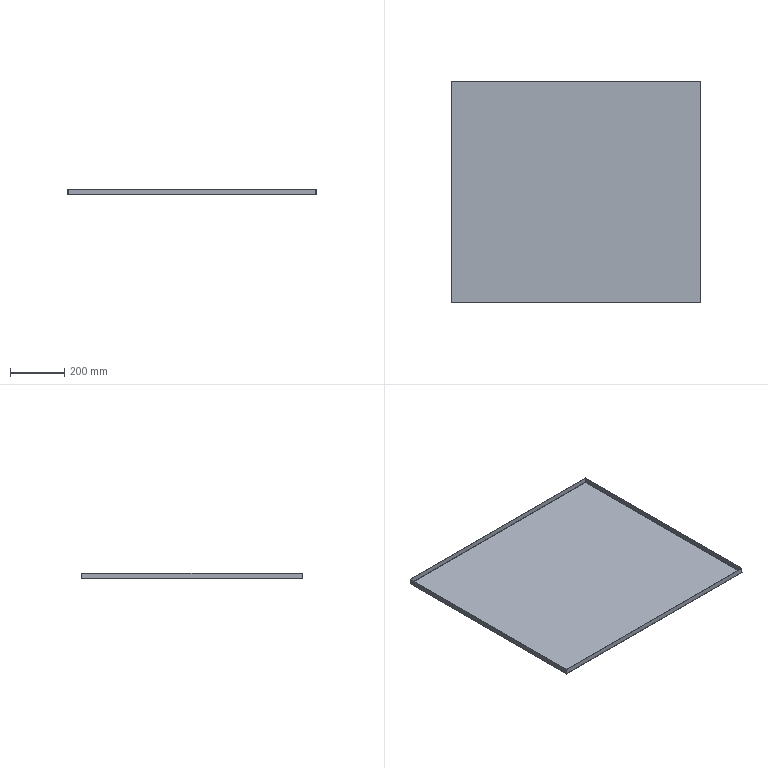Part | STEP file | Cover plate | 1 solid | 38 faces | box 918 x 818 x 20 mm | volume 977655 mm3 | plane 22 | spline 8 | cylinder 8 | commonest cylinder face diameters 0.4 x4 2.8 x4
STEP:
#1=CARTESIAN_POINT('',(457.6,-407.6,-1.2));
#2=VERTEX_POINT('',#1);
#3=CARTESIAN_POINT('',(-457.6,-407.6,-1.2));
#4=VERTEX_POINT('',#3);
#5=CARTESIAN_POINT('',(457.6,-407.6,-1.2));
#6=DIRECTION('',(-1.,0.,0.));
#7=VECTOR('',#6,1000.);
#8=LINE('',#5,#7);
#9=EDGE_CURVE('',#2,#4,#8,.T.);
#10=ORIENTED_EDGE('',*,*,#9,.T.);
#11=CARTESIAN_POINT('',(-457.6,407.6,-1.2));
#12=VERTEX_POINT('',#11);
#13=CARTESIAN_POINT('',(-457.6,-407.6,-1.2));
#14=DIRECTION('',(0.,1.,0.));
#15=VECTOR('',#14,1000.);
#16=LINE('',#13,#15);
#17=EDGE_CURVE('',#4,#12,#16,.T.);
#18=ORIENTED_EDGE('',*,*,#17,.T.);
#19=CARTESIAN_POINT('',(457.6,407.6,-1.2));
#20=VERTEX_POINT('',#19);
#21=CARTESIAN_POINT('',(-457.6,407.6,-1.2));
#22=DIRECTION('',(1.,0.,0.));
#23=VECTOR('',#22,1000.);
#24=LINE('',#21,#23);
#25=EDGE_CURVE('',#12,#20,#24,.T.);
#26=ORIENTED_EDGE('',*,*,#25,.T.);
#27=CARTESIAN_POINT('',(457.6,407.6,-1.2));
#28=DIRECTION('',(0.,-1.,0.));
#29=VECTOR('',#28,1000.);
#30=LINE('',#27,#29);
#31=EDGE_CURVE('',#20,#2,#30,.T.);
#32=ORIENTED_EDGE('',*,*,#31,.T.);
#33=EDGE_LOOP('',(#10,#18,#26,#32));
#34=FACE_OUTER_BOUND('',#33,.T.);
#35=CARTESIAN_POINT('',(0.,0.,-1.2));
#36=DIRECTION('',(0.,0.,-1.));
#37=DIRECTION('',(-1.,0.,0.));
#38=AXIS2_PLACEMENT_3D('',#35,#36,#37);
#39=PLANE('',#38);
#40=ADVANCED_FACE('',(#34),#39,.T.);
#41=CARTESIAN_POINT('',(-457.6,-407.6,0.));
#42=VERTEX_POINT('',#41);
#43=CARTESIAN_POINT('',(-457.6,407.6,0.));
#44=VERTEX_POINT('',#43);
#45=CARTESIAN_POINT('',(-457.6,-407.6,0.));
#46=DIRECTION('',(0.,1.,0.));
#47=VECTOR('',#46,1000.);
#48=LINE('',#45,#47);
#49=EDGE_CURVE('',#42,#44,#48,.T.);
#50=ORIENTED_EDGE('',*,*,#49,.F.);
#51=CARTESIAN_POINT('',(457.6,-407.6,0.));
#52=VERTEX_POINT('',#51);
#53=CARTESIAN_POINT('',(457.6,-407.6,0.));
#54=DIRECTION('',(-1.,0.,0.));
#55=VECTOR('',#54,1000.);
#56=LINE('',#53,#55);
#57=EDGE_CURVE('',#52,#42,#56,.T.);
#58=ORIENTED_EDGE('',*,*,#57,.F.);
#59=CARTESIAN_POINT('',(457.6,407.6,0.));
#60=VERTEX_POINT('',#59);
#61=CARTESIAN_POINT('',(457.6,407.6,0.));
#62=DIRECTION('',(0.,-1.,0.));
#63=VECTOR('',#62,1000.);
#64=LINE('',#61,#63);
#65=EDGE_CURVE('',#60,#52,#64,.T.);
#66=ORIENTED_EDGE('',*,*,#65,.F.);
#67=CARTESIAN_POINT('',(-457.6,407.6,0.));
#68=DIRECTION('',(1.,0.,0.));
#69=VECTOR('',#68,1000.);
#70=LINE('',#67,#69);
#71=EDGE_CURVE('',#44,#60,#70,.T.);
#72=ORIENTED_EDGE('',*,*,#71,.F.);
#73=EDGE_LOOP('',(#50,#58,#66,#72));
#74=FACE_OUTER_BOUND('',#73,.T.);
#75=CARTESIAN_POINT('',(0.,0.,0.));
#76=DIRECTION('',(0.,0.,-1.));
#77=DIRECTION('',(-1.,0.,0.));
#78=AXIS2_PLACEMENT_3D('',#75,#76,#77);
#79=PLANE('',#78);
#80=ADVANCED_FACE('',(#74),#79,.F.);
#81=CARTESIAN_POINT('',(457.093,409.,0.2));
#82=VERTEX_POINT('',#81);
#83=CARTESIAN_POINT('',(457.093,407.8,0.2));
#84=VERTEX_POINT('',#83);
#85=CARTESIAN_POINT('',(457.093,407.8,0.2));
#86=DIRECTION('',(0.,-1.,0.));
#87=VECTOR('',#86,1000.);
#88=LINE('',#85,#87);
#89=EDGE_CURVE('',#82,#84,#88,.T.);
#90=ORIENTED_EDGE('',*,*,#89,.T.);
#91=CARTESIAN_POINT('',(457.6,407.6,0.));
#92=CARTESIAN_POINT('',(457.515,407.652,0.));
#93=CARTESIAN_POINT('',(457.431,407.704,0.02155));
#94=CARTESIAN_POINT('',(457.262,407.778,0.0956));
#95=CARTESIAN_POINT('',(457.177,407.8,0.1476));
#96=CARTESIAN_POINT('',(457.093,407.8,0.2));
#97=B_SPLINE_CURVE_WITH_KNOTS('',3,(#91,#92,#93,#94,#95,#96),.UNSPECIFIED.,.F.,.F.,(4,2,4),(0.,0.5,1.),.UNSPECIFIED.);
#98=EDGE_CURVE('',#60,#84,#97,.T.);
#99=ORIENTED_EDGE('',*,*,#98,.F.);
#100=CARTESIAN_POINT('',(457.6,407.6,0.));
#101=DIRECTION('',(0.,0.,-1.));
#102=VECTOR('',#101,1000.);
#103=LINE('',#100,#102);
#104=EDGE_CURVE('',#60,#20,#103,.T.);
#105=ORIENTED_EDGE('',*,*,#104,.T.);
#106=CARTESIAN_POINT('',(457.6,407.6,-1.2));
#107=CARTESIAN_POINT('',(457.558,407.783,-1.2));
#108=CARTESIAN_POINT('',(457.515,407.966,-1.164));
#109=CARTESIAN_POINT('',(457.431,408.305,-1.023));
#110=CARTESIAN_POINT('',(457.389,408.46,-0.9195));
#111=CARTESIAN_POINT('',(457.304,408.72,-0.6604));
#112=CARTESIAN_POINT('',(457.262,408.823,-0.5051));
#113=CARTESIAN_POINT('',(457.177,408.964,-0.1664));
#114=CARTESIAN_POINT('',(457.135,409.,0.01674));
#115=CARTESIAN_POINT('',(457.093,409.,0.2));
#116=B_SPLINE_CURVE_WITH_KNOTS('',3,(#106,#107,#108,#109,#110,#111,#112,#113,#114,#115),.UNSPECIFIED.,.F.,.F.,(4,2,2,2,4),(0.,0.25,0.5,0.75,1.),.UNSPECIFIED.);
#117=EDGE_CURVE('',#20,#82,#116,.T.);
#118=ORIENTED_EDGE('',*,*,#117,.T.);
#119=EDGE_LOOP('',(#90,#99,#105,#118));
#120=FACE_OUTER_BOUND('',#119,.T.);
#121=CARTESIAN_POINT('',(457.6,407.6,-1.212));
#122=CARTESIAN_POINT('',(457.558,407.785,-1.212));
#123=CARTESIAN_POINT('',(457.515,407.97,-1.175));
#124=CARTESIAN_POINT('',(457.431,408.311,-1.034));
#125=CARTESIAN_POINT('',(457.389,408.468,-0.9291));
#126=CARTESIAN_POINT('',(457.304,408.729,-0.6677));
#127=CARTESIAN_POINT('',(457.262,408.834,-0.5111));
#128=CARTESIAN_POINT('',(457.177,408.975,-0.1696));
#129=CARTESIAN_POINT('',(457.135,409.012,0.01514));
#130=CARTESIAN_POINT('',(457.093,409.012,0.2));
#131=CARTESIAN_POINT('',(457.6,407.6,-1.2));
#132=CARTESIAN_POINT('',(457.558,407.783,-1.2));
#133=CARTESIAN_POINT('',(457.515,407.966,-1.164));
#134=CARTESIAN_POINT('',(457.431,408.305,-1.023));
#135=CARTESIAN_POINT('',(457.389,408.46,-0.9195));
#136=CARTESIAN_POINT('',(457.304,408.72,-0.6604));
#137=CARTESIAN_POINT('',(457.262,408.823,-0.5051));
#138=CARTESIAN_POINT('',(457.177,408.964,-0.1664));
#139=CARTESIAN_POINT('',(457.135,409.,0.01671));
#140=CARTESIAN_POINT('',(457.093,409.,0.2));
#141=CARTESIAN_POINT('',(457.6,407.6,0.));
#142=CARTESIAN_POINT('',(457.558,407.626,0.));
#143=CARTESIAN_POINT('',(457.515,407.652,0.005205));
#144=CARTESIAN_POINT('',(457.431,407.701,0.02524));
#145=CARTESIAN_POINT('',(457.389,407.723,0.04007));
#146=CARTESIAN_POINT('',(457.304,407.76,0.07709));
#147=CARTESIAN_POINT('',(457.262,407.775,0.09928));
#148=CARTESIAN_POINT('',(457.177,407.795,0.1477));
#149=CARTESIAN_POINT('',(457.135,407.8,0.1738));
#150=CARTESIAN_POINT('',(457.093,407.8,0.2));
#151=CARTESIAN_POINT('',(457.6,407.6,0.01212));
#152=CARTESIAN_POINT('',(457.558,407.625,0.01212));
#153=CARTESIAN_POINT('',(457.515,407.649,0.01701));
#154=CARTESIAN_POINT('',(457.431,407.695,0.03583));
#155=CARTESIAN_POINT('',(457.389,407.715,0.04976));
#156=CARTESIAN_POINT('',(457.304,407.75,0.08454));
#157=CARTESIAN_POINT('',(457.262,407.764,0.1054));
#158=CARTESIAN_POINT('',(457.177,407.783,0.1508));
#159=CARTESIAN_POINT('',(457.135,407.788,0.1754));
#160=CARTESIAN_POINT('',(457.093,407.788,0.2));
#161=B_SPLINE_SURFACE_WITH_KNOTS('',1,3,((#121,#122,#123,#124,#125,#126,#127,#128,#129,#130),(#131,#132,#133,#134,#135,#136,#137,#138,#139,#140),(#141,#142,#143,#144,#145,#146,#147,#148,#149,#150),(#151,#152,#153,#154,#155,#156,#157,#158,#159,#160)),.UNSPECIFIED.,.F.,.F.,.F.,(2,1,1,2),(4,2,2,2,4),(-0.01,0.,1.,1.01),(0.,0.25,0.5,0.75,1.),.UNSPECIFIED.);
#162=ADVANCED_FACE('',(#120),#161,.F.);
#163=CARTESIAN_POINT('',(-457.093,407.8,0.2));
#164=VERTEX_POINT('',#163);
#165=CARTESIAN_POINT('',(-457.093,407.8,0.2));
#166=CARTESIAN_POINT('',(-457.177,407.8,0.1476));
#167=CARTESIAN_POINT('',(-457.262,407.778,0.0956));
#168=CARTESIAN_POINT('',(-457.431,407.704,0.02155));
#169=CARTESIAN_POINT('',(-457.515,407.652,0.));
#170=CARTESIAN_POINT('',(-457.6,407.6,0.));
#171=B_SPLINE_CURVE_WITH_KNOTS('',3,(#165,#166,#167,#168,#169,#170),.UNSPECIFIED.,.F.,.F.,(4,2,4),(0.,0.5,1.),.UNSPECIFIED.);
#172=EDGE_CURVE('',#164,#44,#171,.T.);
#173=ORIENTED_EDGE('',*,*,#172,.F.);
#174=CARTESIAN_POINT('',(-457.093,409.,0.2));
#175=VERTEX_POINT('',#174);
#176=CARTESIAN_POINT('',(-457.093,407.8,0.2));
#177=DIRECTION('',(0.,-1.,0.));
#178=VECTOR('',#177,1000.);
#179=LINE('',#176,#178);
#180=EDGE_CURVE('',#175,#164,#179,.T.);
#181=ORIENTED_EDGE('',*,*,#180,.F.);
#182=CARTESIAN_POINT('',(-457.093,409.,0.2));
#183=CARTESIAN_POINT('',(-457.135,409.,0.01674));
#184=CARTESIAN_POINT('',(-457.177,408.964,-0.1664));
#185=CARTESIAN_POINT('',(-457.262,408.823,-0.5051));
#186=CARTESIAN_POINT('',(-457.304,408.72,-0.6604));
#187=CARTESIAN_POINT('',(-457.389,408.46,-0.9195));
#188=CARTESIAN_POINT('',(-457.431,408.305,-1.023));
#189=CARTESIAN_POINT('',(-457.515,407.966,-1.164));
#190=CARTESIAN_POINT('',(-457.558,407.783,-1.2));
#191=CARTESIAN_POINT('',(-457.6,407.6,-1.2));
#192=B_SPLINE_CURVE_WITH_KNOTS('',3,(#182,#183,#184,#185,#186,#187,#188,#189,#190,#191),.UNSPECIFIED.,.F.,.F.,(4,2,2,2,4),(0.,0.25,0.5,0.75,1.),.UNSPECIFIED.);
#193=EDGE_CURVE('',#175,#12,#192,.T.);
#194=ORIENTED_EDGE('',*,*,#193,.T.);
#195=CARTESIAN_POINT('',(-457.6,407.6,0.));
#196=DIRECTION('',(0.,0.,-1.));
#197=VECTOR('',#196,1000.);
#198=LINE('',#195,#197);
#199=EDGE_CURVE('',#44,#12,#198,.T.);
#200=ORIENTED_EDGE('',*,*,#199,.F.);
#201=EDGE_LOOP('',(#173,#181,#194,#200));
#202=FACE_OUTER_BOUND('',#201,.T.);
#203=CARTESIAN_POINT('',(-457.093,409.012,0.2));
#204=CARTESIAN_POINT('',(-457.135,409.012,0.01514));
#205=CARTESIAN_POINT('',(-457.177,408.975,-0.1696));
#206=CARTESIAN_POINT('',(-457.262,408.834,-0.5111));
#207=CARTESIAN_POINT('',(-457.304,408.729,-0.6677));
#208=CARTESIAN_POINT('',(-457.389,408.468,-0.9291));
#209=CARTESIAN_POINT('',(-457.431,408.311,-1.034));
#210=CARTESIAN_POINT('',(-457.515,407.97,-1.175));
#211=CARTESIAN_POINT('',(-457.558,407.785,-1.212));
#212=CARTESIAN_POINT('',(-457.6,407.6,-1.212));
#213=CARTESIAN_POINT('',(-457.093,409.,0.2));
#214=CARTESIAN_POINT('',(-457.135,409.,0.01671));
#215=CARTESIAN_POINT('',(-457.177,408.964,-0.1664));
#216=CARTESIAN_POINT('',(-457.262,408.823,-0.5051));
#217=CARTESIAN_POINT('',(-457.304,408.72,-0.6604));
#218=CARTESIAN_POINT('',(-457.389,408.46,-0.9195));
#219=CARTESIAN_POINT('',(-457.431,408.305,-1.023));
#220=CARTESIAN_POINT('',(-457.515,407.966,-1.164));
#221=CARTESIAN_POINT('',(-457.558,407.783,-1.2));
#222=CARTESIAN_POINT('',(-457.6,407.6,-1.2));
#223=CARTESIAN_POINT('',(-457.093,407.8,0.2));
#224=CARTESIAN_POINT('',(-457.135,407.8,0.1738));
#225=CARTESIAN_POINT('',(-457.177,407.795,0.1477));
#226=CARTESIAN_POINT('',(-457.262,407.775,0.09928));
#227=CARTESIAN_POINT('',(-457.304,407.76,0.07709));
#228=CARTESIAN_POINT('',(-457.389,407.723,0.04007));
#229=CARTESIAN_POINT('',(-457.431,407.701,0.02524));
#230=CARTESIAN_POINT('',(-457.515,407.652,0.005205));
#231=CARTESIAN_POINT('',(-457.558,407.626,0.));
#232=CARTESIAN_POINT('',(-457.6,407.6,0.));
#233=CARTESIAN_POINT('',(-457.093,407.788,0.2));
#234=CARTESIAN_POINT('',(-457.135,407.788,0.1754));
#235=CARTESIAN_POINT('',(-457.177,407.783,0.1508));
#236=CARTESIAN_POINT('',(-457.262,407.764,0.1054));
#237=CARTESIAN_POINT('',(-457.304,407.75,0.08454));
#238=CARTESIAN_POINT('',(-457.389,407.715,0.04976));
#239=CARTESIAN_POINT('',(-457.431,407.695,0.03583));
#240=CARTESIAN_POINT('',(-457.515,407.649,0.01701));
#241=CARTESIAN_POINT('',(-457.558,407.625,0.01212));
#242=CARTESIAN_POINT('',(-457.6,407.6,0.01212));
#243=B_SPLINE_SURFACE_WITH_KNOTS('',1,3,((#203,#204,#205,#206,#207,#208,#209,#210,#211,#212),(#213,#214,#215,#216,#217,#218,#219,#220,#221,#222),(#223,#224,#225,#226,#227,#228,#229,#230,#231,#232),(#233,#234,#235,#236,#237,#238,#239,#240,#241,#242)),.UNSPECIFIED.,.F.,.F.,.F.,(2,1,1,2),(4,2,2,2,4),(-0.01,0.,1.,1.01),(0.,0.25,0.5,0.75,1.),.UNSPECIFIED.);
#244=ADVANCED_FACE('',(#202),#243,.F.);
#245=ORIENTED_EDGE('',*,*,#25,.F.);
#246=ORIENTED_EDGE('',*,*,#193,.F.);
#247=CARTESIAN_POINT('',(459.,409.,0.2));
#248=DIRECTION('',(1.,0.,0.));
#249=VECTOR('',#248,1000.);
#250=LINE('',#247,#249);
#251=EDGE_CURVE('',#175,#82,#250,.T.);
#252=ORIENTED_EDGE('',*,*,#251,.T.);
#253=ORIENTED_EDGE('',*,*,#117,.F.);
#254=EDGE_LOOP('',(#245,#246,#252,#253));
#255=FACE_OUTER_BOUND('',#254,.T.);
#256=CARTESIAN_POINT('',(-457.6,407.6,0.2));
#257=DIRECTION('',(-1.,0.,0.));
#258=DIRECTION('',(0.,1.,0.));
#259=AXIS2_PLACEMENT_3D('',#256,#257,#258);
#260=CYLINDRICAL_SURFACE('',#259,1.4);
#261=ADVANCED_FACE('',(#255),#260,.T.);
#262=ORIENTED_EDGE('',*,*,#71,.T.);
#263=ORIENTED_EDGE('',*,*,#98,.T.);
#264=CARTESIAN_POINT('',(459.,407.8,0.2));
#265=DIRECTION('',(-1.,0.,0.));
#266=VECTOR('',#265,1000.);
#267=LINE('',#264,#266);
#268=EDGE_CURVE('',#84,#164,#267,.T.);
#269=ORIENTED_EDGE('',*,*,#268,.T.);
#270=ORIENTED_EDGE('',*,*,#172,.T.);
#271=EDGE_LOOP('',(#262,#263,#269,#270));
#272=FACE_OUTER_BOUND('',#271,.T.);
#273=CARTESIAN_POINT('',(-457.6,407.6,0.2));
#274=DIRECTION('',(-1.,0.,0.));
#275=DIRECTION('',(0.,1.,0.));
#276=AXIS2_PLACEMENT_3D('',#273,#274,#275);
#277=CYLINDRICAL_SURFACE('',#276,0.2);
#278=ADVANCED_FACE('',(#272),#277,.F.);
#279=CARTESIAN_POINT('',(457.093,409.,18.8));
#280=VERTEX_POINT('',#279);
#281=CARTESIAN_POINT('',(457.093,409.,0.));
#282=DIRECTION('',(0.,0.,1.));
#283=VECTOR('',#282,1000.);
#284=LINE('',#281,#283);
#285=EDGE_CURVE('',#82,#280,#284,.T.);
#286=ORIENTED_EDGE('',*,*,#285,.T.);
#287=CARTESIAN_POINT('',(457.093,407.8,18.8));
#288=VERTEX_POINT('',#287);
#289=CARTESIAN_POINT('',(457.093,407.8,18.8));
#290=DIRECTION('',(0.,-1.,0.));
#291=VECTOR('',#290,1000.);
#292=LINE('',#289,#291);
#293=EDGE_CURVE('',#280,#288,#292,.T.);
#294=ORIENTED_EDGE('',*,*,#293,.T.);
#295=CARTESIAN_POINT('',(457.093,407.8,0.));
#296=DIRECTION('',(0.,0.,1.));
#297=VECTOR('',#296,1000.);
#298=LINE('',#295,#297);
#299=EDGE_CURVE('',#84,#288,#298,.T.);
#300=ORIENTED_EDGE('',*,*,#299,.F.);
#301=ORIENTED_EDGE('',*,*,#89,.F.);
#302=EDGE_LOOP('',(#286,#294,#300,#301));
#303=FACE_OUTER_BOUND('',#302,.T.);
#304=CARTESIAN_POINT('',(457.093,407.8,0.));
#305=DIRECTION('',(1.,0.,0.));
#306=DIRECTION('',(0.,0.,-1.));
#307=AXIS2_PLACEMENT_3D('',#304,#305,#306);
#308=PLANE('',#307);
#309=ADVANCED_FACE('',(#303),#308,.T.);
#310=ORIENTED_EDGE('',*,*,#251,.F.);
#311=CARTESIAN_POINT('',(-457.093,409.,18.8));
#312=VERTEX_POINT('',#311);
#313=CARTESIAN_POINT('',(-457.093,409.,0.));
#314=DIRECTION('',(0.,0.,1.));
#315=VECTOR('',#314,1000.);
#316=LINE('',#313,#315);
#317=EDGE_CURVE('',#175,#312,#316,.T.);
#318=ORIENTED_EDGE('',*,*,#317,.T.);
#319=CARTESIAN_POINT('',(0.,409.,18.8));
#320=DIRECTION('',(1.,0.,0.));
#321=VECTOR('',#320,1000.);
#322=LINE('',#319,#321);
#323=EDGE_CURVE('',#312,#280,#322,.T.);
#324=ORIENTED_EDGE('',*,*,#323,.T.);
#325=ORIENTED_EDGE('',*,*,#285,.F.);
#326=EDGE_LOOP('',(#310,#318,#324,#325));
#327=FACE_OUTER_BOUND('',#326,.T.);
#328=CARTESIAN_POINT('',(0.,409.,0.));
#329=DIRECTION('',(0.,-1.,0.));
#330=DIRECTION('',(0.,0.,-1.));
#331=AXIS2_PLACEMENT_3D('',#328,#329,#330);
#332=PLANE('',#331);
#333=ADVANCED_FACE('',(#327),#332,.F.);
#334=CARTESIAN_POINT('',(-457.093,407.8,18.8));
#335=VERTEX_POINT('',#334);
#336=CARTESIAN_POINT('',(-457.093,407.8,0.));
#337=DIRECTION('',(0.,0.,1.));
#338=VECTOR('',#337,1000.);
#339=LINE('',#336,#338);
#340=EDGE_CURVE('',#164,#335,#339,.T.);
#341=ORIENTED_EDGE('',*,*,#340,.F.);
#342=ORIENTED_EDGE('',*,*,#268,.F.);
#343=ORIENTED_EDGE('',*,*,#299,.T.);
#344=CARTESIAN_POINT('',(459.,407.8,18.8));
#345=DIRECTION('',(1.,0.,0.));
#346=VECTOR('',#345,1000.);
#347=LINE('',#344,#346);
#348=EDGE_CURVE('',#335,#288,#347,.T.);
#349=ORIENTED_EDGE('',*,*,#348,.F.);
#350=EDGE_LOOP('',(#341,#342,#343,#349));
#351=FACE_OUTER_BOUND('',#350,.T.);
#352=CARTESIAN_POINT('',(0.,407.8,0.));
#353=DIRECTION('',(0.,-1.,0.));
#354=DIRECTION('',(0.,0.,-1.));
#355=AXIS2_PLACEMENT_3D('',#352,#353,#354);
#356=PLANE('',#355);
#357=ADVANCED_FACE('',(#351),#356,.T.);
#358=ORIENTED_EDGE('',*,*,#323,.F.);
#359=CARTESIAN_POINT('',(-457.093,409.,18.8));
#360=DIRECTION('',(0.,-1.,0.));
#361=VECTOR('',#360,1000.);
#362=LINE('',#359,#361);
#363=EDGE_CURVE('',#312,#335,#362,.T.);
#364=ORIENTED_EDGE('',*,*,#363,.T.);
#365=ORIENTED_EDGE('',*,*,#348,.T.);
#366=ORIENTED_EDGE('',*,*,#293,.F.);
#367=EDGE_LOOP('',(#358,#364,#365,#366));
#368=FACE_OUTER_BOUND('',#367,.T.);
#369=CARTESIAN_POINT('',(459.,409.,18.8));
#370=DIRECTION('',(0.,0.,-1.));
#371=DIRECTION('',(0.,1.,0.));
#372=AXIS2_PLACEMENT_3D('',#369,#370,#371);
#373=PLANE('',#372);
#374=ADVANCED_FACE('',(#368),#373,.F.);
#375=ORIENTED_EDGE('',*,*,#363,.F.);
#376=ORIENTED_EDGE('',*,*,#317,.F.);
#377=ORIENTED_EDGE('',*,*,#180,.T.);
#378=ORIENTED_EDGE('',*,*,#340,.T.);
#379=EDGE_LOOP('',(#375,#376,#377,#378));
#380=FACE_OUTER_BOUND('',#379,.T.);
#381=CARTESIAN_POINT('',(-457.093,407.8,0.));
#382=DIRECTION('',(1.,0.,0.));
#383=DIRECTION('',(0.,0.,-1.));
#384=AXIS2_PLACEMENT_3D('',#381,#382,#383);
#385=PLANE('',#384);
#386=ADVANCED_FACE('',(#380),#385,.F.);
#387=CARTESIAN_POINT('',(459.,-407.093,0.2));
#388=VERTEX_POINT('',#387);
#389=CARTESIAN_POINT('',(457.8,-407.093,0.2));
#390=VERTEX_POINT('',#389);
#391=CARTESIAN_POINT('',(457.8,-407.093,0.2));
#392=DIRECTION('',(-1.,0.,0.));
#393=VECTOR('',#392,1000.);
#394=LINE('',#391,#393);
#395=EDGE_CURVE('',#388,#390,#394,.T.);
#396=ORIENTED_EDGE('',*,*,#395,.T.);
#397=CARTESIAN_POINT('',(457.6,-407.6,0.));
#398=CARTESIAN_POINT('',(457.652,-407.515,0.));
#399=CARTESIAN_POINT('',(457.704,-407.431,0.02155));
#400=CARTESIAN_POINT('',(457.778,-407.262,0.0956));
#401=CARTESIAN_POINT('',(457.8,-407.177,0.1476));
#402=CARTESIAN_POINT('',(457.8,-407.093,0.2));
#403=B_SPLINE_CURVE_WITH_KNOTS('',3,(#397,#398,#399,#400,#401,#402),.UNSPECIFIED.,.F.,.F.,(4,2,4),(0.,0.5,1.),.UNSPECIFIED.);
#404=EDGE_CURVE('',#52,#390,#403,.T.);
#405=ORIENTED_EDGE('',*,*,#404,.F.);
#406=CARTESIAN_POINT('',(457.6,-407.6,0.));
#407=DIRECTION('',(0.,0.,-1.));
#408=VECTOR('',#407,1000.);
#409=LINE('',#406,#408);
#410=EDGE_CURVE('',#52,#2,#409,.T.);
#411=ORIENTED_EDGE('',*,*,#410,.T.);
#412=CARTESIAN_POINT('',(457.6,-407.6,-1.2));
#413=CARTESIAN_POINT('',(457.783,-407.558,-1.2));
#414=CARTESIAN_POINT('',(457.966,-407.515,-1.164));
#415=CARTESIAN_POINT('',(458.305,-407.431,-1.023));
#416=CARTESIAN_POINT('',(458.46,-407.389,-0.9195));
#417=CARTESIAN_POINT('',(458.72,-407.304,-0.6604));
#418=CARTESIAN_POINT('',(458.823,-407.262,-0.5051));
#419=CARTESIAN_POINT('',(458.964,-407.177,-0.1664));
#420=CARTESIAN_POINT('',(459.,-407.135,0.01674));
#421=CARTESIAN_POINT('',(459.,-407.093,0.2));
#422=B_SPLINE_CURVE_WITH_KNOTS('',3,(#412,#413,#414,#415,#416,#417,#418,#419,#420,#421),.UNSPECIFIED.,.F.,.F.,(4,2,2,2,4),(0.,0.25,0.5,0.75,1.),.UNSPECIFIED.);
#423=EDGE_CURVE('',#2,#388,#422,.T.);
#424=ORIENTED_EDGE('',*,*,#423,.T.);
#425=EDGE_LOOP('',(#396,#405,#411,#424));
#426=FACE_OUTER_BOUND('',#425,.T.);
#427=CARTESIAN_POINT('',(457.6,-407.6,-1.212));
#428=CARTESIAN_POINT('',(457.785,-407.558,-1.212));
#429=CARTESIAN_POINT('',(457.97,-407.515,-1.175));
#430=CARTESIAN_POINT('',(458.311,-407.431,-1.034));
#431=CARTESIAN_POINT('',(458.468,-407.389,-0.9291));
#432=CARTESIAN_POINT('',(458.729,-407.304,-0.6677));
#433=CARTESIAN_POINT('',(458.834,-407.262,-0.5111));
#434=CARTESIAN_POINT('',(458.975,-407.177,-0.1696));
#435=CARTESIAN_POINT('',(459.012,-407.135,0.01514));
#436=CARTESIAN_POINT('',(459.012,-407.093,0.2));
#437=CARTESIAN_POINT('',(457.6,-407.6,-1.2));
#438=CARTESIAN_POINT('',(457.783,-407.558,-1.2));
#439=CARTESIAN_POINT('',(457.966,-407.515,-1.164));
#440=CARTESIAN_POINT('',(458.305,-407.431,-1.023));
#441=CARTESIAN_POINT('',(458.46,-407.389,-0.9195));
#442=CARTESIAN_POINT('',(458.72,-407.304,-0.6604));
#443=CARTESIAN_POINT('',(458.823,-407.262,-0.5051));
#444=CARTESIAN_POINT('',(458.964,-407.177,-0.1664));
#445=CARTESIAN_POINT('',(459.,-407.135,0.01671));
#446=CARTESIAN_POINT('',(459.,-407.093,0.2));
#447=CARTESIAN_POINT('',(457.6,-407.6,0.));
#448=CARTESIAN_POINT('',(457.626,-407.558,0.));
#449=CARTESIAN_POINT('',(457.652,-407.515,0.005205));
#450=CARTESIAN_POINT('',(457.701,-407.431,0.02524));
#451=CARTESIAN_POINT('',(457.723,-407.389,0.04007));
#452=CARTESIAN_POINT('',(457.76,-407.304,0.07709));
#453=CARTESIAN_POINT('',(457.775,-407.262,0.09928));
#454=CARTESIAN_POINT('',(457.795,-407.177,0.1477));
#455=CARTESIAN_POINT('',(457.8,-407.135,0.1738));
#456=CARTESIAN_POINT('',(457.8,-407.093,0.2));
#457=CARTESIAN_POINT('',(457.6,-407.6,0.01212));
#458=CARTESIAN_POINT('',(457.625,-407.558,0.01212));
#459=CARTESIAN_POINT('',(457.649,-407.515,0.01701));
#460=CARTESIAN_POINT('',(457.695,-407.431,0.03583));
#461=CARTESIAN_POINT('',(457.715,-407.389,0.04976));
#462=CARTESIAN_POINT('',(457.75,-407.304,0.08454));
#463=CARTESIAN_POINT('',(457.764,-407.262,0.1054));
#464=CARTESIAN_POINT('',(457.783,-407.177,0.1508));
#465=CARTESIAN_POINT('',(457.788,-407.135,0.1754));
#466=CARTESIAN_POINT('',(457.788,-407.093,0.2));
#467=B_SPLINE_SURFACE_WITH_KNOTS('',1,3,((#427,#428,#429,#430,#431,#432,#433,#434,#435,#436),(#437,#438,#439,#440,#441,#442,#443,#444,#445,#446),(#447,#448,#449,#450,#451,#452,#453,#454,#455,#456),(#457,#458,#459,#460,#461,#462,#463,#464,#465,#466)),.UNSPECIFIED.,.F.,.F.,.F.,(2,1,1,2),(4,2,2,2,4),(-0.01,0.,1.,1.01),(0.,0.25,0.5,0.75,1.),.UNSPECIFIED.);
#468=ADVANCED_FACE('',(#426),#467,.F.);
#469=CARTESIAN_POINT('',(457.8,407.093,0.2));
#470=VERTEX_POINT('',#469);
#471=CARTESIAN_POINT('',(457.8,407.093,0.2));
#472=CARTESIAN_POINT('',(457.8,407.177,0.1476));
#473=CARTESIAN_POINT('',(457.778,407.262,0.0956));
#474=CARTESIAN_POINT('',(457.704,407.431,0.02155));
#475=CARTESIAN_POINT('',(457.652,407.515,0.));
#476=CARTESIAN_POINT('',(457.6,407.6,0.));
#477=B_SPLINE_CURVE_WITH_KNOTS('',3,(#471,#472,#473,#474,#475,#476),.UNSPECIFIED.,.F.,.F.,(4,2,4),(0.,0.5,1.),.UNSPECIFIED.);
#478=EDGE_CURVE('',#470,#60,#477,.T.);
#479=ORIENTED_EDGE('',*,*,#478,.F.);
#480=CARTESIAN_POINT('',(459.,407.093,0.2));
#481=VERTEX_POINT('',#480);
#482=CARTESIAN_POINT('',(457.8,407.093,0.2));
#483=DIRECTION('',(-1.,0.,0.));
#484=VECTOR('',#483,1000.);
#485=LINE('',#482,#484);
#486=EDGE_CURVE('',#481,#470,#485,.T.);
#487=ORIENTED_EDGE('',*,*,#486,.F.);
#488=CARTESIAN_POINT('',(459.,407.093,0.2));
#489=CARTESIAN_POINT('',(459.,407.135,0.01674));
#490=CARTESIAN_POINT('',(458.964,407.177,-0.1664));
#491=CARTESIAN_POINT('',(458.823,407.262,-0.5051));
#492=CARTESIAN_POINT('',(458.72,407.304,-0.6604));
#493=CARTESIAN_POINT('',(458.46,407.389,-0.9195));
#494=CARTESIAN_POINT('',(458.305,407.431,-1.023));
#495=CARTESIAN_POINT('',(457.966,407.515,-1.164));
#496=CARTESIAN_POINT('',(457.783,407.558,-1.2));
#497=CARTESIAN_POINT('',(457.6,407.6,-1.2));
#498=B_SPLINE_CURVE_WITH_KNOTS('',3,(#488,#489,#490,#491,#492,#493,#494,#495,#496,#497),.UNSPECIFIED.,.F.,.F.,(4,2,2,2,4),(0.,0.25,0.5,0.75,1.),.UNSPECIFIED.);
#499=EDGE_CURVE('',#481,#20,#498,.T.);
#500=ORIENTED_EDGE('',*,*,#499,.T.);
#501=ORIENTED_EDGE('',*,*,#104,.F.);
#502=EDGE_LOOP('',(#479,#487,#500,#501));
#503=FACE_OUTER_BOUND('',#502,.T.);
#504=CARTESIAN_POINT('',(459.012,407.093,0.2));
#505=CARTESIAN_POINT('',(459.012,407.135,0.01514));
#506=CARTESIAN_POINT('',(458.975,407.177,-0.1696));
#507=CARTESIAN_POINT('',(458.834,407.262,-0.5111));
#508=CARTESIAN_POINT('',(458.729,407.304,-0.6677));
#509=CARTESIAN_POINT('',(458.468,407.389,-0.9291));
#510=CARTESIAN_POINT('',(458.311,407.431,-1.034));
#511=CARTESIAN_POINT('',(457.97,407.515,-1.175));
#512=CARTESIAN_POINT('',(457.785,407.558,-1.212));
#513=CARTESIAN_POINT('',(457.6,407.6,-1.212));
#514=CARTESIAN_POINT('',(459.,407.093,0.2));
#515=CARTESIAN_POINT('',(459.,407.135,0.01671));
#516=CARTESIAN_POINT('',(458.964,407.177,-0.1664));
#517=CARTESIAN_POINT('',(458.823,407.262,-0.5051));
#518=CARTESIAN_POINT('',(458.72,407.304,-0.6604));
#519=CARTESIAN_POINT('',(458.46,407.389,-0.9195));
#520=CARTESIAN_POINT('',(458.305,407.431,-1.023));
#521=CARTESIAN_POINT('',(457.966,407.515,-1.164));
#522=CARTESIAN_POINT('',(457.783,407.558,-1.2));
#523=CARTESIAN_POINT('',(457.6,407.6,-1.2));
#524=CARTESIAN_POINT('',(457.8,407.093,0.2));
#525=CARTESIAN_POINT('',(457.8,407.135,0.1738));
#526=CARTESIAN_POINT('',(457.795,407.177,0.1477));
#527=CARTESIAN_POINT('',(457.775,407.262,0.09928));
#528=CARTESIAN_POINT('',(457.76,407.304,0.07709));
#529=CARTESIAN_POINT('',(457.723,407.389,0.04007));
#530=CARTESIAN_POINT('',(457.701,407.431,0.02524));
#531=CARTESIAN_POINT('',(457.652,407.515,0.005205));
#532=CARTESIAN_POINT('',(457.626,407.558,0.));
#533=CARTESIAN_POINT('',(457.6,407.6,0.));
#534=CARTESIAN_POINT('',(457.788,407.093,0.2));
#535=CARTESIAN_POINT('',(457.788,407.135,0.1754));
#536=CARTESIAN_POINT('',(457.783,407.177,0.1508));
#537=CARTESIAN_POINT('',(457.764,407.262,0.1054));
#538=CARTESIAN_POINT('',(457.75,407.304,0.08454));
#539=CARTESIAN_POINT('',(457.715,407.389,0.04976));
#540=CARTESIAN_POINT('',(457.695,407.431,0.03583));
#541=CARTESIAN_POINT('',(457.649,407.515,0.01701));
#542=CARTESIAN_POINT('',(457.625,407.558,0.01212));
#543=CARTESIAN_POINT('',(457.6,407.6,0.01212));
#544=B_SPLINE_SURFACE_WITH_KNOTS('',1,3,((#504,#505,#506,#507,#508,#509,#510,#511,#512,#513),(#514,#515,#516,#517,#518,#519,#520,#521,#522,#523),(#524,#525,#526,#527,#528,#529,#530,#531,#532,#533),(#534,#535,#536,#537,#538,#539,#540,#541,#542,#543)),.UNSPECIFIED.,.F.,.F.,.F.,(2,1,1,2),(4,2,2,2,4),(-0.01,0.,1.,1.01),(0.,0.25,0.5,0.75,1.),.UNSPECIFIED.);
#545=ADVANCED_FACE('',(#503),#544,.F.);
#546=ORIENTED_EDGE('',*,*,#31,.F.);
#547=ORIENTED_EDGE('',*,*,#499,.F.);
#548=CARTESIAN_POINT('',(459.,-409.,0.2));
#549=DIRECTION('',(0.,-1.,0.));
#550=VECTOR('',#549,1000.);
#551=LINE('',#548,#550);
#552=EDGE_CURVE('',#481,#388,#551,.T.);
#553=ORIENTED_EDGE('',*,*,#552,.T.);
#554=ORIENTED_EDGE('',*,*,#423,.F.);
#555=EDGE_LOOP('',(#546,#547,#553,#554));
#556=FACE_OUTER_BOUND('',#555,.T.);
#557=CARTESIAN_POINT('',(457.6,407.6,0.2));
#558=DIRECTION('',(0.,1.,0.));
#559=DIRECTION('',(1.,0.,0.));
#560=AXIS2_PLACEMENT_3D('',#557,#558,#559);
#561=CYLINDRICAL_SURFACE('',#560,1.4);
#562=ADVANCED_FACE('',(#556),#561,.T.);
#563=ORIENTED_EDGE('',*,*,#65,.T.);
#564=ORIENTED_EDGE('',*,*,#404,.T.);
#565=CARTESIAN_POINT('',(457.8,-409.,0.2));
#566=DIRECTION('',(0.,1.,0.));
#567=VECTOR('',#566,1000.);
#568=LINE('',#565,#567);
#569=EDGE_CURVE('',#390,#470,#568,.T.);
#570=ORIENTED_EDGE('',*,*,#569,.T.);
#571=ORIENTED_EDGE('',*,*,#478,.T.);
#572=EDGE_LOOP('',(#563,#564,#570,#571));
#573=FACE_OUTER_BOUND('',#572,.T.);
#574=CARTESIAN_POINT('',(457.6,407.6,0.2));
#575=DIRECTION('',(0.,1.,0.));
#576=DIRECTION('',(1.,0.,0.));
#577=AXIS2_PLACEMENT_3D('',#574,#575,#576);
#578=CYLINDRICAL_SURFACE('',#577,0.2);
#579=ADVANCED_FACE('',(#573),#578,.F.);
#580=CARTESIAN_POINT('',(459.,-407.093,18.8));
#581=VERTEX_POINT('',#580);
#582=CARTESIAN_POINT('',(459.,-407.093,0.));
#583=DIRECTION('',(0.,0.,1.));
#584=VECTOR('',#583,1000.);
#585=LINE('',#582,#584);
#586=EDGE_CURVE('',#388,#581,#585,.T.);
#587=ORIENTED_EDGE('',*,*,#586,.T.);
#588=CARTESIAN_POINT('',(457.8,-407.093,18.8));
#589=VERTEX_POINT('',#588);
#590=CARTESIAN_POINT('',(457.8,-407.093,18.8));
#591=DIRECTION('',(-1.,0.,0.));
#592=VECTOR('',#591,1000.);
#593=LINE('',#590,#592);
#594=EDGE_CURVE('',#581,#589,#593,.T.);
#595=ORIENTED_EDGE('',*,*,#594,.T.);
#596=CARTESIAN_POINT('',(457.8,-407.093,0.));
#597=DIRECTION('',(0.,0.,1.));
#598=VECTOR('',#597,1000.);
#599=LINE('',#596,#598);
#600=EDGE_CURVE('',#390,#589,#599,.T.);
#601=ORIENTED_EDGE('',*,*,#600,.F.);
#602=ORIENTED_EDGE('',*,*,#395,.F.);
#603=EDGE_LOOP('',(#587,#595,#601,#602));
#604=FACE_OUTER_BOUND('',#603,.T.);
#605=CARTESIAN_POINT('',(457.8,-407.093,0.));
#606=DIRECTION('',(0.,-1.,0.));
#607=DIRECTION('',(0.,0.,-1.));
#608=AXIS2_PLACEMENT_3D('',#605,#606,#607);
#609=PLANE('',#608);
#610=ADVANCED_FACE('',(#604),#609,.T.);
#611=ORIENTED_EDGE('',*,*,#552,.F.);
#612=CARTESIAN_POINT('',(459.,407.093,18.8));
#613=VERTEX_POINT('',#612);
#614=CARTESIAN_POINT('',(459.,407.093,0.));
#615=DIRECTION('',(0.,0.,1.));
#616=VECTOR('',#615,1000.);
#617=LINE('',#614,#616);
#618=EDGE_CURVE('',#481,#613,#617,.T.);
#619=ORIENTED_EDGE('',*,*,#618,.T.);
#620=CARTESIAN_POINT('',(459.,0.,18.8));
#621=DIRECTION('',(0.,-1.,0.));
#622=VECTOR('',#621,1000.);
#623=LINE('',#620,#622);
#624=EDGE_CURVE('',#613,#581,#623,.T.);
#625=ORIENTED_EDGE('',*,*,#624,.T.);
#626=ORIENTED_EDGE('',*,*,#586,.F.);
#627=EDGE_LOOP('',(#611,#619,#625,#626));
#628=FACE_OUTER_BOUND('',#627,.T.);
#629=CARTESIAN_POINT('',(459.,0.,0.));
#630=DIRECTION('',(-1.,0.,0.));
#631=DIRECTION('',(0.,0.,1.));
#632=AXIS2_PLACEMENT_3D('',#629,#630,#631);
#633=PLANE('',#632);
#634=ADVANCED_FACE('',(#628),#633,.F.);
#635=CARTESIAN_POINT('',(457.8,407.093,18.8));
#636=VERTEX_POINT('',#635);
#637=CARTESIAN_POINT('',(457.8,407.093,0.));
#638=DIRECTION('',(0.,0.,1.));
#639=VECTOR('',#638,1000.);
#640=LINE('',#637,#639);
#641=EDGE_CURVE('',#470,#636,#640,.T.);
#642=ORIENTED_EDGE('',*,*,#641,.F.);
#643=ORIENTED_EDGE('',*,*,#569,.F.);
#644=ORIENTED_EDGE('',*,*,#600,.T.);
#645=CARTESIAN_POINT('',(457.8,-409.,18.8));
#646=DIRECTION('',(0.,-1.,0.));
#647=VECTOR('',#646,1000.);
#648=LINE('',#645,#647);
#649=EDGE_CURVE('',#636,#589,#648,.T.);
#650=ORIENTED_EDGE('',*,*,#649,.F.);
#651=EDGE_LOOP('',(#642,#643,#644,#650));
#652=FACE_OUTER_BOUND('',#651,.T.);
#653=CARTESIAN_POINT('',(457.8,0.,0.));
#654=DIRECTION('',(-1.,0.,0.));
#655=DIRECTION('',(0.,0.,1.));
#656=AXIS2_PLACEMENT_3D('',#653,#654,#655);
#657=PLANE('',#656);
#658=ADVANCED_FACE('',(#652),#657,.T.);
#659=ORIENTED_EDGE('',*,*,#624,.F.);
#660=CARTESIAN_POINT('',(459.,407.093,18.8));
#661=DIRECTION('',(-1.,0.,0.));
#662=VECTOR('',#661,1000.);
#663=LINE('',#660,#662);
#664=EDGE_CURVE('',#613,#636,#663,.T.);
#665=ORIENTED_EDGE('',*,*,#664,.T.);
#666=ORIENTED_EDGE('',*,*,#649,.T.);
#667=ORIENTED_EDGE('',*,*,#594,.F.);
#668=EDGE_LOOP('',(#659,#665,#666,#667));
#669=FACE_OUTER_BOUND('',#668,.T.);
#670=CARTESIAN_POINT('',(459.,-409.,18.8));
#671=DIRECTION('',(0.,0.,-1.));
#672=DIRECTION('',(-1.,0.,0.));
#673=AXIS2_PLACEMENT_3D('',#670,#671,#672);
#674=PLANE('',#673);
#675=ADVANCED_FACE('',(#669),#674,.F.);
#676=ORIENTED_EDGE('',*,*,#664,.F.);
#677=ORIENTED_EDGE('',*,*,#618,.F.);
#678=ORIENTED_EDGE('',*,*,#486,.T.);
#679=ORIENTED_EDGE('',*,*,#641,.T.);
#680=EDGE_LOOP('',(#676,#677,#678,#679));
#681=FACE_OUTER_BOUND('',#680,.T.);
#682=CARTESIAN_POINT('',(457.8,407.093,0.));
#683=DIRECTION('',(0.,-1.,0.));
#684=DIRECTION('',(0.,0.,-1.));
#685=AXIS2_PLACEMENT_3D('',#682,#683,#684);
#686=PLANE('',#685);
#687=ADVANCED_FACE('',(#681),#686,.F.);
#688=CARTESIAN_POINT('',(-457.093,-409.,0.2));
#689=VERTEX_POINT('',#688);
#690=CARTESIAN_POINT('',(-457.093,-407.8,0.2));
#691=VERTEX_POINT('',#690);
#692=CARTESIAN_POINT('',(-457.093,-407.8,0.2));
#693=DIRECTION('',(0.,1.,0.));
#694=VECTOR('',#693,1000.);
#695=LINE('',#692,#694);
#696=EDGE_CURVE('',#689,#691,#695,.T.);
#697=ORIENTED_EDGE('',*,*,#696,.T.);
#698=CARTESIAN_POINT('',(-457.6,-407.6,0.));
#699=CARTESIAN_POINT('',(-457.515,-407.652,0.));
#700=CARTESIAN_POINT('',(-457.431,-407.704,0.02155));
#701=CARTESIAN_POINT('',(-457.262,-407.778,0.0956));
#702=CARTESIAN_POINT('',(-457.177,-407.8,0.1476));
#703=CARTESIAN_POINT('',(-457.093,-407.8,0.2));
#704=B_SPLINE_CURVE_WITH_KNOTS('',3,(#698,#699,#700,#701,#702,#703),.UNSPECIFIED.,.F.,.F.,(4,2,4),(0.,0.5,1.),.UNSPECIFIED.);
#705=EDGE_CURVE('',#42,#691,#704,.T.);
#706=ORIENTED_EDGE('',*,*,#705,.F.);
#707=CARTESIAN_POINT('',(-457.6,-407.6,0.));
#708=DIRECTION('',(0.,0.,-1.));
#709=VECTOR('',#708,1000.);
#710=LINE('',#707,#709);
#711=EDGE_CURVE('',#42,#4,#710,.T.);
#712=ORIENTED_EDGE('',*,*,#711,.T.);
#713=CARTESIAN_POINT('',(-457.6,-407.6,-1.2));
#714=CARTESIAN_POINT('',(-457.558,-407.783,-1.2));
#715=CARTESIAN_POINT('',(-457.515,-407.966,-1.164));
#716=CARTESIAN_POINT('',(-457.431,-408.305,-1.023));
#717=CARTESIAN_POINT('',(-457.389,-408.46,-0.9195));
#718=CARTESIAN_POINT('',(-457.304,-408.72,-0.6604));
#719=CARTESIAN_POINT('',(-457.262,-408.823,-0.5051));
#720=CARTESIAN_POINT('',(-457.177,-408.964,-0.1664));
#721=CARTESIAN_POINT('',(-457.135,-409.,0.01674));
#722=CARTESIAN_POINT('',(-457.093,-409.,0.2));
#723=B_SPLINE_CURVE_WITH_KNOTS('',3,(#713,#714,#715,#716,#717,#718,#719,#720,#721,#722),.UNSPECIFIED.,.F.,.F.,(4,2,2,2,4),(0.,0.25,0.5,0.75,1.),.UNSPECIFIED.);
#724=EDGE_CURVE('',#4,#689,#723,.T.);
#725=ORIENTED_EDGE('',*,*,#724,.T.);
#726=EDGE_LOOP('',(#697,#706,#712,#725));
#727=FACE_OUTER_BOUND('',#726,.T.);
#728=CARTESIAN_POINT('',(-457.6,-407.6,-1.212));
#729=CARTESIAN_POINT('',(-457.558,-407.785,-1.212));
#730=CARTESIAN_POINT('',(-457.515,-407.97,-1.175));
#731=CARTESIAN_POINT('',(-457.431,-408.311,-1.034));
#732=CARTESIAN_POINT('',(-457.389,-408.468,-0.9291));
#733=CARTESIAN_POINT('',(-457.304,-408.729,-0.6677));
#734=CARTESIAN_POINT('',(-457.262,-408.834,-0.5111));
#735=CARTESIAN_POINT('',(-457.177,-408.975,-0.1696));
#736=CARTESIAN_POINT('',(-457.135,-409.012,0.01514));
#737=CARTESIAN_POINT('',(-457.093,-409.012,0.2));
#738=CARTESIAN_POINT('',(-457.6,-407.6,-1.2));
#739=CARTESIAN_POINT('',(-457.558,-407.783,-1.2));
#740=CARTESIAN_POINT('',(-457.515,-407.966,-1.164));
#741=CARTESIAN_POINT('',(-457.431,-408.305,-1.023));
#742=CARTESIAN_POINT('',(-457.389,-408.46,-0.9195));
#743=CARTESIAN_POINT('',(-457.304,-408.72,-0.6604));
#744=CARTESIAN_POINT('',(-457.262,-408.823,-0.5051));
#745=CARTESIAN_POINT('',(-457.177,-408.964,-0.1664));
#746=CARTESIAN_POINT('',(-457.135,-409.,0.01671));
#747=CARTESIAN_POINT('',(-457.093,-409.,0.2));
#748=CARTESIAN_POINT('',(-457.6,-407.6,0.));
#749=CARTESIAN_POINT('',(-457.558,-407.626,0.));
#750=CARTESIAN_POINT('',(-457.515,-407.652,0.005205));
#751=CARTESIAN_POINT('',(-457.431,-407.701,0.02524));
#752=CARTESIAN_POINT('',(-457.389,-407.723,0.04007));
#753=CARTESIAN_POINT('',(-457.304,-407.76,0.07709));
#754=CARTESIAN_POINT('',(-457.262,-407.775,0.09928));
#755=CARTESIAN_POINT('',(-457.177,-407.795,0.1477));
#756=CARTESIAN_POINT('',(-457.135,-407.8,0.1738));
#757=CARTESIAN_POINT('',(-457.093,-407.8,0.2));
#758=CARTESIAN_POINT('',(-457.6,-407.6,0.01212));
#759=CARTESIAN_POINT('',(-457.558,-407.625,0.01212));
#760=CARTESIAN_POINT('',(-457.515,-407.649,0.01701));
#761=CARTESIAN_POINT('',(-457.431,-407.695,0.03583));
#762=CARTESIAN_POINT('',(-457.389,-407.715,0.04976));
#763=CARTESIAN_POINT('',(-457.304,-407.75,0.08454));
#764=CARTESIAN_POINT('',(-457.262,-407.764,0.1054));
#765=CARTESIAN_POINT('',(-457.177,-407.783,0.1508));
#766=CARTESIAN_POINT('',(-457.135,-407.788,0.1754));
#767=CARTESIAN_POINT('',(-457.093,-407.788,0.2));
#768=B_SPLINE_SURFACE_WITH_KNOTS('',1,3,((#728,#729,#730,#731,#732,#733,#734,#735,#736,#737),(#738,#739,#740,#741,#742,#743,#744,#745,#746,#747),(#748,#749,#750,#751,#752,#753,#754,#755,#756,#757),(#758,#759,#760,#761,#762,#763,#764,#765,#766,#767)),.UNSPECIFIED.,.F.,.F.,.F.,(2,1,1,2),(4,2,2,2,4),(-0.01,0.,1.,1.01),(0.,0.25,0.5,0.75,1.),.UNSPECIFIED.);
#769=ADVANCED_FACE('',(#727),#768,.F.);
#770=CARTESIAN_POINT('',(457.093,-407.8,0.2));
#771=VERTEX_POINT('',#770);
#772=CARTESIAN_POINT('',(457.093,-407.8,0.2));
#773=CARTESIAN_POINT('',(457.177,-407.8,0.1476));
#774=CARTESIAN_POINT('',(457.262,-407.778,0.0956));
#775=CARTESIAN_POINT('',(457.431,-407.704,0.02155));
#776=CARTESIAN_POINT('',(457.515,-407.652,0.));
#777=CARTESIAN_POINT('',(457.6,-407.6,0.));
#778=B_SPLINE_CURVE_WITH_KNOTS('',3,(#772,#773,#774,#775,#776,#777),.UNSPECIFIED.,.F.,.F.,(4,2,4),(0.,0.5,1.),.UNSPECIFIED.);
#779=EDGE_CURVE('',#771,#52,#778,.T.);
#780=ORIENTED_EDGE('',*,*,#779,.F.);
#781=CARTESIAN_POINT('',(457.093,-409.,0.2));
#782=VERTEX_POINT('',#781);
#783=CARTESIAN_POINT('',(457.093,-407.8,0.2));
#784=DIRECTION('',(0.,1.,0.));
#785=VECTOR('',#784,1000.);
#786=LINE('',#783,#785);
#787=EDGE_CURVE('',#782,#771,#786,.T.);
#788=ORIENTED_EDGE('',*,*,#787,.F.);
#789=CARTESIAN_POINT('',(457.093,-409.,0.2));
#790=CARTESIAN_POINT('',(457.135,-409.,0.01674));
#791=CARTESIAN_POINT('',(457.177,-408.964,-0.1664));
#792=CARTESIAN_POINT('',(457.262,-408.823,-0.5051));
#793=CARTESIAN_POINT('',(457.304,-408.72,-0.6604));
#794=CARTESIAN_POINT('',(457.389,-408.46,-0.9195));
#795=CARTESIAN_POINT('',(457.431,-408.305,-1.023));
#796=CARTESIAN_POINT('',(457.515,-407.966,-1.164));
#797=CARTESIAN_POINT('',(457.558,-407.783,-1.2));
#798=CARTESIAN_POINT('',(457.6,-407.6,-1.2));
#799=B_SPLINE_CURVE_WITH_KNOTS('',3,(#789,#790,#791,#792,#793,#794,#795,#796,#797,#798),.UNSPECIFIED.,.F.,.F.,(4,2,2,2,4),(0.,0.25,0.5,0.75,1.),.UNSPECIFIED.);
#800=EDGE_CURVE('',#782,#2,#799,.T.);
#801=ORIENTED_EDGE('',*,*,#800,.T.);
#802=ORIENTED_EDGE('',*,*,#410,.F.);
#803=EDGE_LOOP('',(#780,#788,#801,#802));
#804=FACE_OUTER_BOUND('',#803,.T.);
#805=CARTESIAN_POINT('',(457.093,-409.012,0.2));
#806=CARTESIAN_POINT('',(457.135,-409.012,0.01514));
#807=CARTESIAN_POINT('',(457.177,-408.975,-0.1696));
#808=CARTESIAN_POINT('',(457.262,-408.834,-0.5111));
#809=CARTESIAN_POINT('',(457.304,-408.729,-0.6677));
#810=CARTESIAN_POINT('',(457.389,-408.468,-0.9291));
#811=CARTESIAN_POINT('',(457.431,-408.311,-1.034));
#812=CARTESIAN_POINT('',(457.515,-407.97,-1.175));
#813=CARTESIAN_POINT('',(457.558,-407.785,-1.212));
#814=CARTESIAN_POINT('',(457.6,-407.6,-1.212));
#815=CARTESIAN_POINT('',(457.093,-409.,0.2));
#816=CARTESIAN_POINT('',(457.135,-409.,0.01671));
#817=CARTESIAN_POINT('',(457.177,-408.964,-0.1664));
#818=CARTESIAN_POINT('',(457.262,-408.823,-0.5051));
#819=CARTESIAN_POINT('',(457.304,-408.72,-0.6604));
#820=CARTESIAN_POINT('',(457.389,-408.46,-0.9195));
#821=CARTESIAN_POINT('',(457.431,-408.305,-1.023));
#822=CARTESIAN_POINT('',(457.515,-407.966,-1.164));
#823=CARTESIAN_POINT('',(457.558,-407.783,-1.2));
#824=CARTESIAN_POINT('',(457.6,-407.6,-1.2));
#825=CARTESIAN_POINT('',(457.093,-407.8,0.2));
#826=CARTESIAN_POINT('',(457.135,-407.8,0.1738));
#827=CARTESIAN_POINT('',(457.177,-407.795,0.1477));
#828=CARTESIAN_POINT('',(457.262,-407.775,0.09928));
#829=CARTESIAN_POINT('',(457.304,-407.76,0.07709));
#830=CARTESIAN_POINT('',(457.389,-407.723,0.04007));
#831=CARTESIAN_POINT('',(457.431,-407.701,0.02524));
#832=CARTESIAN_POINT('',(457.515,-407.652,0.005205));
#833=CARTESIAN_POINT('',(457.558,-407.626,0.));
#834=CARTESIAN_POINT('',(457.6,-407.6,0.));
#835=CARTESIAN_POINT('',(457.093,-407.788,0.2));
#836=CARTESIAN_POINT('',(457.135,-407.788,0.1754));
#837=CARTESIAN_POINT('',(457.177,-407.783,0.1508));
#838=CARTESIAN_POINT('',(457.262,-407.764,0.1054));
#839=CARTESIAN_POINT('',(457.304,-407.75,0.08454));
#840=CARTESIAN_POINT('',(457.389,-407.715,0.04976));
#841=CARTESIAN_POINT('',(457.431,-407.695,0.03583));
#842=CARTESIAN_POINT('',(457.515,-407.649,0.01701));
#843=CARTESIAN_POINT('',(457.558,-407.625,0.01212));
#844=CARTESIAN_POINT('',(457.6,-407.6,0.01212));
#845=B_SPLINE_SURFACE_WITH_KNOTS('',1,3,((#805,#806,#807,#808,#809,#810,#811,#812,#813,#814),(#815,#816,#817,#818,#819,#820,#821,#822,#823,#824),(#825,#826,#827,#828,#829,#830,#831,#832,#833,#834),(#835,#836,#837,#838,#839,#840,#841,#842,#843,#844)),.UNSPECIFIED.,.F.,.F.,.F.,(2,1,1,2),(4,2,2,2,4),(-0.01,0.,1.,1.01),(0.,0.25,0.5,0.75,1.),.UNSPECIFIED.);
#846=ADVANCED_FACE('',(#804),#845,.F.);
#847=ORIENTED_EDGE('',*,*,#9,.F.);
#848=ORIENTED_EDGE('',*,*,#800,.F.);
#849=CARTESIAN_POINT('',(-459.,-409.,0.2));
#850=DIRECTION('',(-1.,0.,0.));
#851=VECTOR('',#850,1000.);
#852=LINE('',#849,#851);
#853=EDGE_CURVE('',#782,#689,#852,.T.);
#854=ORIENTED_EDGE('',*,*,#853,.T.);
#855=ORIENTED_EDGE('',*,*,#724,.F.);
#856=EDGE_LOOP('',(#847,#848,#854,#855));
#857=FACE_OUTER_BOUND('',#856,.T.);
#858=CARTESIAN_POINT('',(457.6,-407.6,0.2));
#859=DIRECTION('',(1.,0.,0.));
#860=DIRECTION('',(0.,-1.,0.));
#861=AXIS2_PLACEMENT_3D('',#858,#859,#860);
#862=CYLINDRICAL_SURFACE('',#861,1.4);
#863=ADVANCED_FACE('',(#857),#862,.T.);
#864=ORIENTED_EDGE('',*,*,#57,.T.);
#865=ORIENTED_EDGE('',*,*,#705,.T.);
#866=CARTESIAN_POINT('',(-459.,-407.8,0.2));
#867=DIRECTION('',(1.,0.,0.));
#868=VECTOR('',#867,1000.);
#869=LINE('',#866,#868);
#870=EDGE_CURVE('',#691,#771,#869,.T.);
#871=ORIENTED_EDGE('',*,*,#870,.T.);
#872=ORIENTED_EDGE('',*,*,#779,.T.);
#873=EDGE_LOOP('',(#864,#865,#871,#872));
#874=FACE_OUTER_BOUND('',#873,.T.);
#875=CARTESIAN_POINT('',(457.6,-407.6,0.2));
#876=DIRECTION('',(1.,0.,0.));
#877=DIRECTION('',(0.,-1.,0.));
#878=AXIS2_PLACEMENT_3D('',#875,#876,#877);
#879=CYLINDRICAL_SURFACE('',#878,0.2);
#880=ADVANCED_FACE('',(#874),#879,.F.);
#881=CARTESIAN_POINT('',(-457.093,-409.,18.8));
#882=VERTEX_POINT('',#881);
#883=CARTESIAN_POINT('',(-457.093,-409.,0.));
#884=DIRECTION('',(0.,0.,1.));
#885=VECTOR('',#884,1000.);
#886=LINE('',#883,#885);
#887=EDGE_CURVE('',#689,#882,#886,.T.);
#888=ORIENTED_EDGE('',*,*,#887,.T.);
#889=CARTESIAN_POINT('',(-457.093,-407.8,18.8));
#890=VERTEX_POINT('',#889);
#891=CARTESIAN_POINT('',(-457.093,-407.8,18.8));
#892=DIRECTION('',(0.,1.,0.));
#893=VECTOR('',#892,1000.);
#894=LINE('',#891,#893);
#895=EDGE_CURVE('',#882,#890,#894,.T.);
#896=ORIENTED_EDGE('',*,*,#895,.T.);
#897=CARTESIAN_POINT('',(-457.093,-407.8,0.));
#898=DIRECTION('',(0.,0.,1.));
#899=VECTOR('',#898,1000.);
#900=LINE('',#897,#899);
#901=EDGE_CURVE('',#691,#890,#900,.T.);
#902=ORIENTED_EDGE('',*,*,#901,.F.);
#903=ORIENTED_EDGE('',*,*,#696,.F.);
#904=EDGE_LOOP('',(#888,#896,#902,#903));
#905=FACE_OUTER_BOUND('',#904,.T.);
#906=CARTESIAN_POINT('',(-457.093,-407.8,0.));
#907=DIRECTION('',(-1.,0.,0.));
#908=DIRECTION('',(0.,0.,1.));
#909=AXIS2_PLACEMENT_3D('',#906,#907,#908);
#910=PLANE('',#909);
#911=ADVANCED_FACE('',(#905),#910,.T.);
#912=ORIENTED_EDGE('',*,*,#853,.F.);
#913=CARTESIAN_POINT('',(457.093,-409.,18.8));
#914=VERTEX_POINT('',#913);
#915=CARTESIAN_POINT('',(457.093,-409.,0.));
#916=DIRECTION('',(0.,0.,1.));
#917=VECTOR('',#916,1000.);
#918=LINE('',#915,#917);
#919=EDGE_CURVE('',#782,#914,#918,.T.);
#920=ORIENTED_EDGE('',*,*,#919,.T.);
#921=CARTESIAN_POINT('',(0.,-409.,18.8));
#922=DIRECTION('',(-1.,0.,0.));
#923=VECTOR('',#922,1000.);
#924=LINE('',#921,#923);
#925=EDGE_CURVE('',#914,#882,#924,.T.);
#926=ORIENTED_EDGE('',*,*,#925,.T.);
#927=ORIENTED_EDGE('',*,*,#887,.F.);
#928=EDGE_LOOP('',(#912,#920,#926,#927));
#929=FACE_OUTER_BOUND('',#928,.T.);
#930=CARTESIAN_POINT('',(0.,-409.,0.));
#931=DIRECTION('',(0.,1.,0.));
#932=DIRECTION('',(0.,0.,1.));
#933=AXIS2_PLACEMENT_3D('',#930,#931,#932);
#934=PLANE('',#933);
#935=ADVANCED_FACE('',(#929),#934,.F.);
#936=CARTESIAN_POINT('',(457.093,-407.8,18.8));
#937=VERTEX_POINT('',#936);
#938=CARTESIAN_POINT('',(457.093,-407.8,0.));
#939=DIRECTION('',(0.,0.,1.));
#940=VECTOR('',#939,1000.);
#941=LINE('',#938,#940);
#942=EDGE_CURVE('',#771,#937,#941,.T.);
#943=ORIENTED_EDGE('',*,*,#942,.F.);
#944=ORIENTED_EDGE('',*,*,#870,.F.);
#945=ORIENTED_EDGE('',*,*,#901,.T.);
#946=CARTESIAN_POINT('',(-459.,-407.8,18.8));
#947=DIRECTION('',(-1.,0.,0.));
#948=VECTOR('',#947,1000.);
#949=LINE('',#946,#948);
#950=EDGE_CURVE('',#937,#890,#949,.T.);
#951=ORIENTED_EDGE('',*,*,#950,.F.);
#952=EDGE_LOOP('',(#943,#944,#945,#951));
#953=FACE_OUTER_BOUND('',#952,.T.);
#954=CARTESIAN_POINT('',(0.,-407.8,0.));
#955=DIRECTION('',(0.,1.,0.));
#956=DIRECTION('',(0.,0.,1.));
#957=AXIS2_PLACEMENT_3D('',#954,#955,#956);
#958=PLANE('',#957);
#959=ADVANCED_FACE('',(#953),#958,.T.);
#960=ORIENTED_EDGE('',*,*,#925,.F.);
#961=CARTESIAN_POINT('',(457.093,-409.,18.8));
#962=DIRECTION('',(0.,1.,0.));
#963=VECTOR('',#962,1000.);
#964=LINE('',#961,#963);
#965=EDGE_CURVE('',#914,#937,#964,.T.);
#966=ORIENTED_EDGE('',*,*,#965,.T.);
#967=ORIENTED_EDGE('',*,*,#950,.T.);
#968=ORIENTED_EDGE('',*,*,#895,.F.);
#969=EDGE_LOOP('',(#960,#966,#967,#968));
#970=FACE_OUTER_BOUND('',#969,.T.);
#971=CARTESIAN_POINT('',(-459.,-409.,18.8));
#972=DIRECTION('',(0.,0.,-1.));
#973=DIRECTION('',(0.,1.,0.));
#974=AXIS2_PLACEMENT_3D('',#971,#972,#973);
#975=PLANE('',#974);
#976=ADVANCED_FACE('',(#970),#975,.F.);
#977=ORIENTED_EDGE('',*,*,#965,.F.);
#978=ORIENTED_EDGE('',*,*,#919,.F.);
#979=ORIENTED_EDGE('',*,*,#787,.T.);
#980=ORIENTED_EDGE('',*,*,#942,.T.);
#981=EDGE_LOOP('',(#977,#978,#979,#980));
#982=FACE_OUTER_BOUND('',#981,.T.);
#983=CARTESIAN_POINT('',(457.093,-407.8,0.));
#984=DIRECTION('',(-1.,0.,0.));
#985=DIRECTION('',(0.,0.,1.));
#986=AXIS2_PLACEMENT_3D('',#983,#984,#985);
#987=PLANE('',#986);
#988=ADVANCED_FACE('',(#982),#987,.F.);
#989=CARTESIAN_POINT('',(-459.,407.093,0.2));
#990=VERTEX_POINT('',#989);
#991=CARTESIAN_POINT('',(-457.8,407.093,0.2));
#992=VERTEX_POINT('',#991);
#993=CARTESIAN_POINT('',(-457.8,407.093,0.2));
#994=DIRECTION('',(1.,0.,0.));
#995=VECTOR('',#994,1000.);
#996=LINE('',#993,#995);
#997=EDGE_CURVE('',#990,#992,#996,.T.);
#998=ORIENTED_EDGE('',*,*,#997,.T.);
#999=CARTESIAN_POINT('',(-457.6,407.6,0.));
#1000=CARTESIAN_POINT('',(-457.652,407.515,0.));
#1001=CARTESIAN_POINT('',(-457.704,407.431,0.02155));
#1002=CARTESIAN_POINT('',(-457.778,407.262,0.0956));
#1003=CARTESIAN_POINT('',(-457.8,407.177,0.1476));
#1004=CARTESIAN_POINT('',(-457.8,407.093,0.2));
#1005=B_SPLINE_CURVE_WITH_KNOTS('',3,(#999,#1000,#1001,#1002,#1003,#1004),.UNSPECIFIED.,.F.,.F.,(4,2,4),(0.,0.5,1.),.UNSPECIFIED.);
#1006=EDGE_CURVE('',#44,#992,#1005,.T.);
#1007=ORIENTED_EDGE('',*,*,#1006,.F.);
#1008=ORIENTED_EDGE('',*,*,#199,.T.);
#1009=CARTESIAN_POINT('',(-457.6,407.6,-1.2));
#1010=CARTESIAN_POINT('',(-457.783,407.558,-1.2));
#1011=CARTESIAN_POINT('',(-457.966,407.515,-1.164));
#1012=CARTESIAN_POINT('',(-458.305,407.431,-1.023));
#1013=CARTESIAN_POINT('',(-458.46,407.389,-0.9195));
#1014=CARTESIAN_POINT('',(-458.72,407.304,-0.6604));
#1015=CARTESIAN_POINT('',(-458.823,407.262,-0.5051));
#1016=CARTESIAN_POINT('',(-458.964,407.177,-0.1664));
#1017=CARTESIAN_POINT('',(-459.,407.135,0.01674));
#1018=CARTESIAN_POINT('',(-459.,407.093,0.2));
#1019=B_SPLINE_CURVE_WITH_KNOTS('',3,(#1009,#1010,#1011,#1012,#1013,#1014,#1015,#1016,#1017,#1018),.UNSPECIFIED.,.F.,.F.,(4,2,2,2,4),(0.,0.25,0.5,0.75,1.),.UNSPECIFIED.);
#1020=EDGE_CURVE('',#12,#990,#1019,.T.);
#1021=ORIENTED_EDGE('',*,*,#1020,.T.);
#1022=EDGE_LOOP('',(#998,#1007,#1008,#1021));
#1023=FACE_OUTER_BOUND('',#1022,.T.);
#1024=CARTESIAN_POINT('',(-457.6,407.6,-1.212));
#1025=CARTESIAN_POINT('',(-457.785,407.558,-1.212));
#1026=CARTESIAN_POINT('',(-457.97,407.515,-1.175));
#1027=CARTESIAN_POINT('',(-458.311,407.431,-1.034));
#1028=CARTESIAN_POINT('',(-458.468,407.389,-0.9291));
#1029=CARTESIAN_POINT('',(-458.729,407.304,-0.6677));
#1030=CARTESIAN_POINT('',(-458.834,407.262,-0.5111));
#1031=CARTESIAN_POINT('',(-458.975,407.177,-0.1696));
#1032=CARTESIAN_POINT('',(-459.012,407.135,0.01514));
#1033=CARTESIAN_POINT('',(-459.012,407.093,0.2));
#1034=CARTESIAN_POINT('',(-457.6,407.6,-1.2));
#1035=CARTESIAN_POINT('',(-457.783,407.558,-1.2));
#1036=CARTESIAN_POINT('',(-457.966,407.515,-1.164));
#1037=CARTESIAN_POINT('',(-458.305,407.431,-1.023));
#1038=CARTESIAN_POINT('',(-458.46,407.389,-0.9195));
#1039=CARTESIAN_POINT('',(-458.72,407.304,-0.6604));
#1040=CARTESIAN_POINT('',(-458.823,407.262,-0.5051));
#1041=CARTESIAN_POINT('',(-458.964,407.177,-0.1664));
#1042=CARTESIAN_POINT('',(-459.,407.135,0.01671));
#1043=CARTESIAN_POINT('',(-459.,407.093,0.2));
#1044=CARTESIAN_POINT('',(-457.6,407.6,0.));
#1045=CARTESIAN_POINT('',(-457.626,407.558,0.));
#1046=CARTESIAN_POINT('',(-457.652,407.515,0.005205));
#1047=CARTESIAN_POINT('',(-457.701,407.431,0.02524));
#1048=CARTESIAN_POINT('',(-457.723,407.389,0.04007));
#1049=CARTESIAN_POINT('',(-457.76,407.304,0.07709));
#1050=CARTESIAN_POINT('',(-457.775,407.262,0.09928));
#1051=CARTESIAN_POINT('',(-457.795,407.177,0.1477));
#1052=CARTESIAN_POINT('',(-457.8,407.135,0.1738));
#1053=CARTESIAN_POINT('',(-457.8,407.093,0.2));
#1054=CARTESIAN_POINT('',(-457.6,407.6,0.01212));
#1055=CARTESIAN_POINT('',(-457.625,407.558,0.01212));
#1056=CARTESIAN_POINT('',(-457.649,407.515,0.01701));
#1057=CARTESIAN_POINT('',(-457.695,407.431,0.03583));
#1058=CARTESIAN_POINT('',(-457.715,407.389,0.04976));
#1059=CARTESIAN_POINT('',(-457.75,407.304,0.08454));
#1060=CARTESIAN_POINT('',(-457.764,407.262,0.1054));
#1061=CARTESIAN_POINT('',(-457.783,407.177,0.1508));
#1062=CARTESIAN_POINT('',(-457.788,407.135,0.1754));
#1063=CARTESIAN_POINT('',(-457.788,407.093,0.2));
#1064=B_SPLINE_SURFACE_WITH_KNOTS('',1,3,((#1024,#1025,#1026,#1027,#1028,#1029,#1030,#1031,#1032,#1033),(#1034,#1035,#1036,#1037,#1038,#1039,#1040,#1041,#1042,#1043),(#1044,#1045,#1046,#1047,#1048,#1049,#1050,#1051,#1052,#1053),(#1054,#1055,#1056,#1057,#1058,#1059,#1060,#1061,#1062,#1063)),.UNSPECIFIED.,.F.,.F.,.F.,(2,1,1,2),(4,2,2,2,4),(-0.01,0.,1.,1.01),(0.,0.25,0.5,0.75,1.),.UNSPECIFIED.);
#1065=ADVANCED_FACE('',(#1023),#1064,.F.);
#1066=CARTESIAN_POINT('',(-457.8,-407.093,0.2));
#1067=VERTEX_POINT('',#1066);
#1068=CARTESIAN_POINT('',(-457.8,-407.093,0.2));
#1069=CARTESIAN_POINT('',(-457.8,-407.177,0.1476));
#1070=CARTESIAN_POINT('',(-457.778,-407.262,0.0956));
#1071=CARTESIAN_POINT('',(-457.704,-407.431,0.02155));
#1072=CARTESIAN_POINT('',(-457.652,-407.515,0.));
#1073=CARTESIAN_POINT('',(-457.6,-407.6,0.));
#1074=B_SPLINE_CURVE_WITH_KNOTS('',3,(#1068,#1069,#1070,#1071,#1072,#1073),.UNSPECIFIED.,.F.,.F.,(4,2,4),(0.,0.5,1.),.UNSPECIFIED.);
#1075=EDGE_CURVE('',#1067,#42,#1074,.T.);
#1076=ORIENTED_EDGE('',*,*,#1075,.F.);
#1077=CARTESIAN_POINT('',(-459.,-407.093,0.2));
#1078=VERTEX_POINT('',#1077);
#1079=CARTESIAN_POINT('',(-457.8,-407.093,0.2));
#1080=DIRECTION('',(1.,0.,0.));
#1081=VECTOR('',#1080,1000.);
#1082=LINE('',#1079,#1081);
#1083=EDGE_CURVE('',#1078,#1067,#1082,.T.);
#1084=ORIENTED_EDGE('',*,*,#1083,.F.);
#1085=CARTESIAN_POINT('',(-459.,-407.093,0.2));
#1086=CARTESIAN_POINT('',(-459.,-407.135,0.01674));
#1087=CARTESIAN_POINT('',(-458.964,-407.177,-0.1664));
#1088=CARTESIAN_POINT('',(-458.823,-407.262,-0.5051));
#1089=CARTESIAN_POINT('',(-458.72,-407.304,-0.6604));
#1090=CARTESIAN_POINT('',(-458.46,-407.389,-0.9195));
#1091=CARTESIAN_POINT('',(-458.305,-407.431,-1.023));
#1092=CARTESIAN_POINT('',(-457.966,-407.515,-1.164));
#1093=CARTESIAN_POINT('',(-457.783,-407.558,-1.2));
#1094=CARTESIAN_POINT('',(-457.6,-407.6,-1.2));
#1095=B_SPLINE_CURVE_WITH_KNOTS('',3,(#1085,#1086,#1087,#1088,#1089,#1090,#1091,#1092,#1093,#1094),.UNSPECIFIED.,.F.,.F.,(4,2,2,2,4),(0.,0.25,0.5,0.75,1.),.UNSPECIFIED.);
#1096=EDGE_CURVE('',#1078,#4,#1095,.T.);
#1097=ORIENTED_EDGE('',*,*,#1096,.T.);
#1098=ORIENTED_EDGE('',*,*,#711,.F.);
#1099=EDGE_LOOP('',(#1076,#1084,#1097,#1098));
#1100=FACE_OUTER_BOUND('',#1099,.T.);
#1101=CARTESIAN_POINT('',(-459.012,-407.093,0.2));
#1102=CARTESIAN_POINT('',(-459.012,-407.135,0.01514));
#1103=CARTESIAN_POINT('',(-458.975,-407.177,-0.1696));
#1104=CARTESIAN_POINT('',(-458.834,-407.262,-0.5111));
#1105=CARTESIAN_POINT('',(-458.729,-407.304,-0.6677));
#1106=CARTESIAN_POINT('',(-458.468,-407.389,-0.9291));
#1107=CARTESIAN_POINT('',(-458.311,-407.431,-1.034));
#1108=CARTESIAN_POINT('',(-457.97,-407.515,-1.175));
#1109=CARTESIAN_POINT('',(-457.785,-407.558,-1.212));
#1110=CARTESIAN_POINT('',(-457.6,-407.6,-1.212));
#1111=CARTESIAN_POINT('',(-459.,-407.093,0.2));
#1112=CARTESIAN_POINT('',(-459.,-407.135,0.01671));
#1113=CARTESIAN_POINT('',(-458.964,-407.177,-0.1664));
#1114=CARTESIAN_POINT('',(-458.823,-407.262,-0.5051));
#1115=CARTESIAN_POINT('',(-458.72,-407.304,-0.6604));
#1116=CARTESIAN_POINT('',(-458.46,-407.389,-0.9195));
#1117=CARTESIAN_POINT('',(-458.305,-407.431,-1.023));
#1118=CARTESIAN_POINT('',(-457.966,-407.515,-1.164));
#1119=CARTESIAN_POINT('',(-457.783,-407.558,-1.2));
#1120=CARTESIAN_POINT('',(-457.6,-407.6,-1.2));
#1121=CARTESIAN_POINT('',(-457.8,-407.093,0.2));
#1122=CARTESIAN_POINT('',(-457.8,-407.135,0.1738));
#1123=CARTESIAN_POINT('',(-457.795,-407.177,0.1477));
#1124=CARTESIAN_POINT('',(-457.775,-407.262,0.09928));
#1125=CARTESIAN_POINT('',(-457.76,-407.304,0.07709));
#1126=CARTESIAN_POINT('',(-457.723,-407.389,0.04007));
#1127=CARTESIAN_POINT('',(-457.701,-407.431,0.02524));
#1128=CARTESIAN_POINT('',(-457.652,-407.515,0.005205));
#1129=CARTESIAN_POINT('',(-457.626,-407.558,0.));
#1130=CARTESIAN_POINT('',(-457.6,-407.6,0.));
#1131=CARTESIAN_POINT('',(-457.788,-407.093,0.2));
#1132=CARTESIAN_POINT('',(-457.788,-407.135,0.1754));
#1133=CARTESIAN_POINT('',(-457.783,-407.177,0.1508));
#1134=CARTESIAN_POINT('',(-457.764,-407.262,0.1054));
#1135=CARTESIAN_POINT('',(-457.75,-407.304,0.08454));
#1136=CARTESIAN_POINT('',(-457.715,-407.389,0.04976));
#1137=CARTESIAN_POINT('',(-457.695,-407.431,0.03583));
#1138=CARTESIAN_POINT('',(-457.649,-407.515,0.01701));
#1139=CARTESIAN_POINT('',(-457.625,-407.558,0.01212));
#1140=CARTESIAN_POINT('',(-457.6,-407.6,0.01212));
#1141=B_SPLINE_SURFACE_WITH_KNOTS('',1,3,((#1101,#1102,#1103,#1104,#1105,#1106,#1107,#1108,#1109,#1110),(#1111,#1112,#1113,#1114,#1115,#1116,#1117,#1118,#1119,#1120),(#1121,#1122,#1123,#1124,#1125,#1126,#1127,#1128,#1129,#1130),(#1131,#1132,#1133,#1134,#1135,#1136,#1137,#1138,#1139,#1140)),.UNSPECIFIED.,.F.,.F.,.F.,(2,1,1,2),(4,2,2,2,4),(-0.01,0.,1.,1.01),(0.,0.25,0.5,0.75,1.),.UNSPECIFIED.);
#1142=ADVANCED_FACE('',(#1100),#1141,.F.);
#1143=ORIENTED_EDGE('',*,*,#17,.F.);
#1144=ORIENTED_EDGE('',*,*,#1096,.F.);
#1145=CARTESIAN_POINT('',(-459.,409.,0.2));
#1146=DIRECTION('',(0.,1.,0.));
#1147=VECTOR('',#1146,1000.);
#1148=LINE('',#1145,#1147);
#1149=EDGE_CURVE('',#1078,#990,#1148,.T.);
#1150=ORIENTED_EDGE('',*,*,#1149,.T.);
#1151=ORIENTED_EDGE('',*,*,#1020,.F.);
#1152=EDGE_LOOP('',(#1143,#1144,#1150,#1151));
#1153=FACE_OUTER_BOUND('',#1152,.T.);
#1154=CARTESIAN_POINT('',(-457.6,-407.6,0.2));
#1155=DIRECTION('',(0.,-1.,0.));
#1156=DIRECTION('',(-1.,0.,0.));
#1157=AXIS2_PLACEMENT_3D('',#1154,#1155,#1156);
#1158=CYLINDRICAL_SURFACE('',#1157,1.4);
#1159=ADVANCED_FACE('',(#1153),#1158,.T.);
#1160=ORIENTED_EDGE('',*,*,#49,.T.);
#1161=ORIENTED_EDGE('',*,*,#1006,.T.);
#1162=CARTESIAN_POINT('',(-457.8,409.,0.2));
#1163=DIRECTION('',(0.,-1.,0.));
#1164=VECTOR('',#1163,1000.);
#1165=LINE('',#1162,#1164);
#1166=EDGE_CURVE('',#992,#1067,#1165,.T.);
#1167=ORIENTED_EDGE('',*,*,#1166,.T.);
#1168=ORIENTED_EDGE('',*,*,#1075,.T.);
#1169=EDGE_LOOP('',(#1160,#1161,#1167,#1168));
#1170=FACE_OUTER_BOUND('',#1169,.T.);
#1171=CARTESIAN_POINT('',(-457.6,-407.6,0.2));
#1172=DIRECTION('',(0.,-1.,0.));
#1173=DIRECTION('',(-1.,0.,0.));
#1174=AXIS2_PLACEMENT_3D('',#1171,#1172,#1173);
#1175=CYLINDRICAL_SURFACE('',#1174,0.2);
#1176=ADVANCED_FACE('',(#1170),#1175,.F.);
#1177=CARTESIAN_POINT('',(-459.,407.093,18.8));
#1178=VERTEX_POINT('',#1177);
#1179=CARTESIAN_POINT('',(-459.,407.093,0.));
#1180=DIRECTION('',(0.,0.,1.));
#1181=VECTOR('',#1180,1000.);
#1182=LINE('',#1179,#1181);
#1183=EDGE_CURVE('',#990,#1178,#1182,.T.);
#1184=ORIENTED_EDGE('',*,*,#1183,.T.);
#1185=CARTESIAN_POINT('',(-457.8,407.093,18.8));
#1186=VERTEX_POINT('',#1185);
#1187=CARTESIAN_POINT('',(-457.8,407.093,18.8));
#1188=DIRECTION('',(1.,0.,0.));
#1189=VECTOR('',#1188,1000.);
#1190=LINE('',#1187,#1189);
#1191=EDGE_CURVE('',#1178,#1186,#1190,.T.);
#1192=ORIENTED_EDGE('',*,*,#1191,.T.);
#1193=CARTESIAN_POINT('',(-457.8,407.093,0.));
#1194=DIRECTION('',(0.,0.,1.));
#1195=VECTOR('',#1194,1000.);
#1196=LINE('',#1193,#1195);
#1197=EDGE_CURVE('',#992,#1186,#1196,.T.);
#1198=ORIENTED_EDGE('',*,*,#1197,.F.);
#1199=ORIENTED_EDGE('',*,*,#997,.F.);
#1200=EDGE_LOOP('',(#1184,#1192,#1198,#1199));
#1201=FACE_OUTER_BOUND('',#1200,.T.);
#1202=CARTESIAN_POINT('',(-457.8,407.093,0.));
#1203=DIRECTION('',(0.,1.,0.));
#1204=DIRECTION('',(0.,0.,1.));
#1205=AXIS2_PLACEMENT_3D('',#1202,#1203,#1204);
#1206=PLANE('',#1205);
#1207=ADVANCED_FACE('',(#1201),#1206,.T.);
#1208=ORIENTED_EDGE('',*,*,#1149,.F.);
#1209=CARTESIAN_POINT('',(-459.,-407.093,18.8));
#1210=VERTEX_POINT('',#1209);
#1211=CARTESIAN_POINT('',(-459.,-407.093,0.));
#1212=DIRECTION('',(0.,0.,1.));
#1213=VECTOR('',#1212,1000.);
#1214=LINE('',#1211,#1213);
#1215=EDGE_CURVE('',#1078,#1210,#1214,.T.);
#1216=ORIENTED_EDGE('',*,*,#1215,.T.);
#1217=CARTESIAN_POINT('',(-459.,0.,18.8));
#1218=DIRECTION('',(0.,1.,0.));
#1219=VECTOR('',#1218,1000.);
#1220=LINE('',#1217,#1219);
#1221=EDGE_CURVE('',#1210,#1178,#1220,.T.);
#1222=ORIENTED_EDGE('',*,*,#1221,.T.);
#1223=ORIENTED_EDGE('',*,*,#1183,.F.);
#1224=EDGE_LOOP('',(#1208,#1216,#1222,#1223));
#1225=FACE_OUTER_BOUND('',#1224,.T.);
#1226=CARTESIAN_POINT('',(-459.,0.,0.));
#1227=DIRECTION('',(1.,0.,0.));
#1228=DIRECTION('',(0.,0.,-1.));
#1229=AXIS2_PLACEMENT_3D('',#1226,#1227,#1228);
#1230=PLANE('',#1229);
#1231=ADVANCED_FACE('',(#1225),#1230,.F.);
#1232=CARTESIAN_POINT('',(-457.8,-407.093,18.8));
#1233=VERTEX_POINT('',#1232);
#1234=CARTESIAN_POINT('',(-457.8,-407.093,0.));
#1235=DIRECTION('',(0.,0.,1.));
#1236=VECTOR('',#1235,1000.);
#1237=LINE('',#1234,#1236);
#1238=EDGE_CURVE('',#1067,#1233,#1237,.T.);
#1239=ORIENTED_EDGE('',*,*,#1238,.F.);
#1240=ORIENTED_EDGE('',*,*,#1166,.F.);
#1241=ORIENTED_EDGE('',*,*,#1197,.T.);
#1242=CARTESIAN_POINT('',(-457.8,409.,18.8));
#1243=DIRECTION('',(0.,1.,0.));
#1244=VECTOR('',#1243,1000.);
#1245=LINE('',#1242,#1244);
#1246=EDGE_CURVE('',#1233,#1186,#1245,.T.);
#1247=ORIENTED_EDGE('',*,*,#1246,.F.);
#1248=EDGE_LOOP('',(#1239,#1240,#1241,#1247));
#1249=FACE_OUTER_BOUND('',#1248,.T.);
#1250=CARTESIAN_POINT('',(-457.8,0.,0.));
#1251=DIRECTION('',(1.,0.,0.));
#1252=DIRECTION('',(0.,0.,-1.));
#1253=AXIS2_PLACEMENT_3D('',#1250,#1251,#1252);
#1254=PLANE('',#1253);
#1255=ADVANCED_FACE('',(#1249),#1254,.T.);
#1256=ORIENTED_EDGE('',*,*,#1221,.F.);
#1257=CARTESIAN_POINT('',(-459.,-407.093,18.8));
#1258=DIRECTION('',(1.,0.,0.));
#1259=VECTOR('',#1258,1000.);
#1260=LINE('',#1257,#1259);
#1261=EDGE_CURVE('',#1210,#1233,#1260,.T.);
#1262=ORIENTED_EDGE('',*,*,#1261,.T.);
#1263=ORIENTED_EDGE('',*,*,#1246,.T.);
#1264=ORIENTED_EDGE('',*,*,#1191,.F.);
#1265=EDGE_LOOP('',(#1256,#1262,#1263,#1264));
#1266=FACE_OUTER_BOUND('',#1265,.T.);
#1267=CARTESIAN_POINT('',(-459.,409.,18.8));
#1268=DIRECTION('',(0.,0.,-1.));
#1269=DIRECTION('',(-1.,0.,0.));
#1270=AXIS2_PLACEMENT_3D('',#1267,#1268,#1269);
#1271=PLANE('',#1270);
#1272=ADVANCED_FACE('',(#1266),#1271,.F.);
#1273=ORIENTED_EDGE('',*,*,#1261,.F.);
#1274=ORIENTED_EDGE('',*,*,#1215,.F.);
#1275=ORIENTED_EDGE('',*,*,#1083,.T.);
#1276=ORIENTED_EDGE('',*,*,#1238,.T.);
#1277=EDGE_LOOP('',(#1273,#1274,#1275,#1276));
#1278=FACE_OUTER_BOUND('',#1277,.T.);
#1279=CARTESIAN_POINT('',(-457.8,-407.093,0.));
#1280=DIRECTION('',(0.,1.,0.));
#1281=DIRECTION('',(0.,0.,1.));
#1282=AXIS2_PLACEMENT_3D('',#1279,#1280,#1281);
#1283=PLANE('',#1282);
#1284=ADVANCED_FACE('',(#1278),#1283,.F.);
#1285=CLOSED_SHELL('',(#40,#80,#162,#244,#261,#278,#309,#333,#357,#374,#386,#468,#545,#562,#579,#610,#634,#658,#675,#687,#769,#846,#863,#880,#911,#935,#959,#976,#988,#1065,#1142,#1159,#1176,#1207,#1231,#1255,#1272,#1284));
#1286=MANIFOLD_SOLID_BREP('',#1285);
#1287=CARTESIAN_POINT('',(0.,0.,0.));
#1288=DIRECTION('',(0.,0.,1.));
#1289=DIRECTION('',(1.,0.,0.));
#1290=AXIS2_PLACEMENT_3D('',#1287,#1288,#1289);
#1291=(LENGTH_UNIT()NAMED_UNIT(*)SI_UNIT(.MILLI.,.METRE.));
#1292=UNCERTAINTY_MEASURE_WITH_UNIT(LENGTH_MEASURE(0.00001),#1291,'','');
#1293=(NAMED_UNIT(*)PLANE_ANGLE_UNIT()SI_UNIT($,.RADIAN.));
#1294=(NAMED_UNIT(*)SI_UNIT($,.STERADIAN.)SOLID_ANGLE_UNIT());
#1295=(GEOMETRIC_REPRESENTATION_CONTEXT(3)GLOBAL_UNCERTAINTY_ASSIGNED_CONTEXT((#1292))GLOBAL_UNIT_ASSIGNED_CONTEXT((#1291,#1293,#1294))REPRESENTATION_CONTEXT('',''));
#1296=ADVANCED_BREP_SHAPE_REPRESENTATION('',(#1286,#1290),#1295);